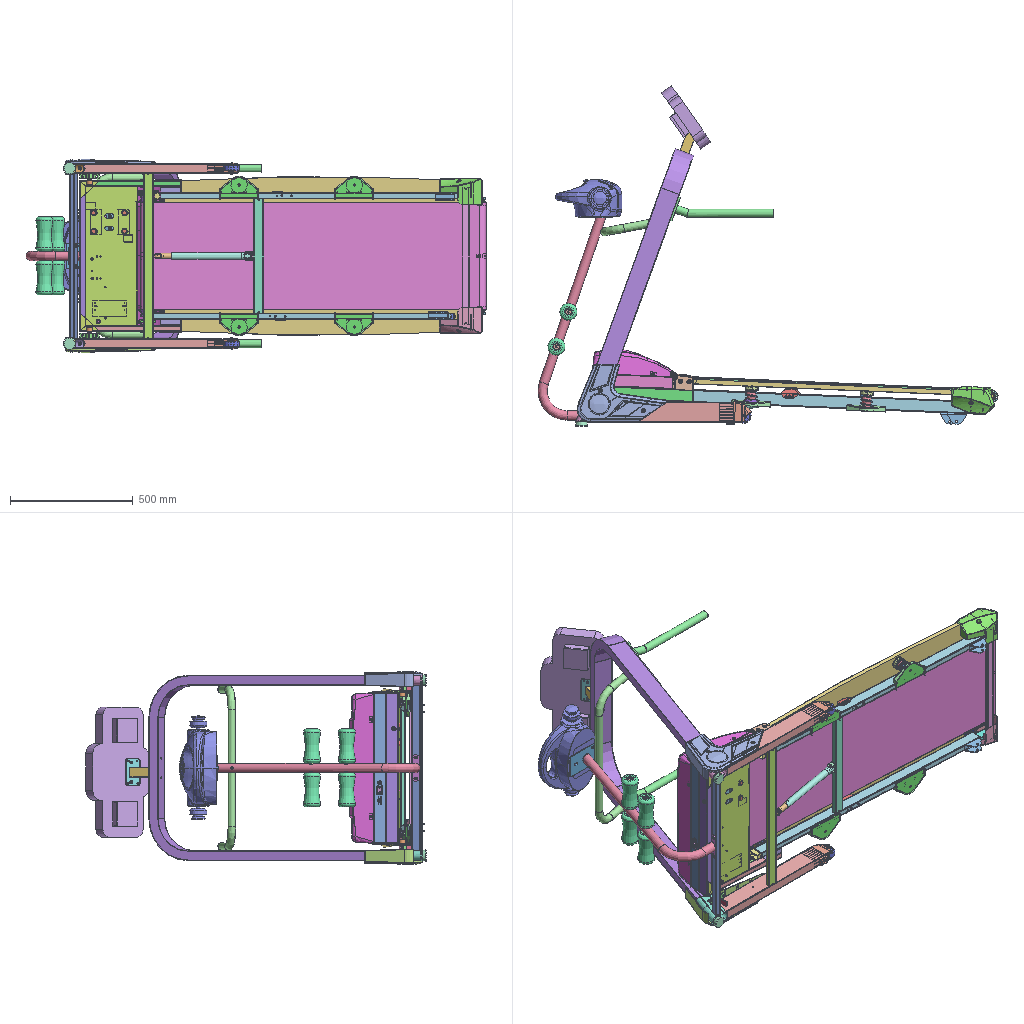Assembly | STEP file | 111 different items | 206 placed | box 1875 x 1387 x 788 mm
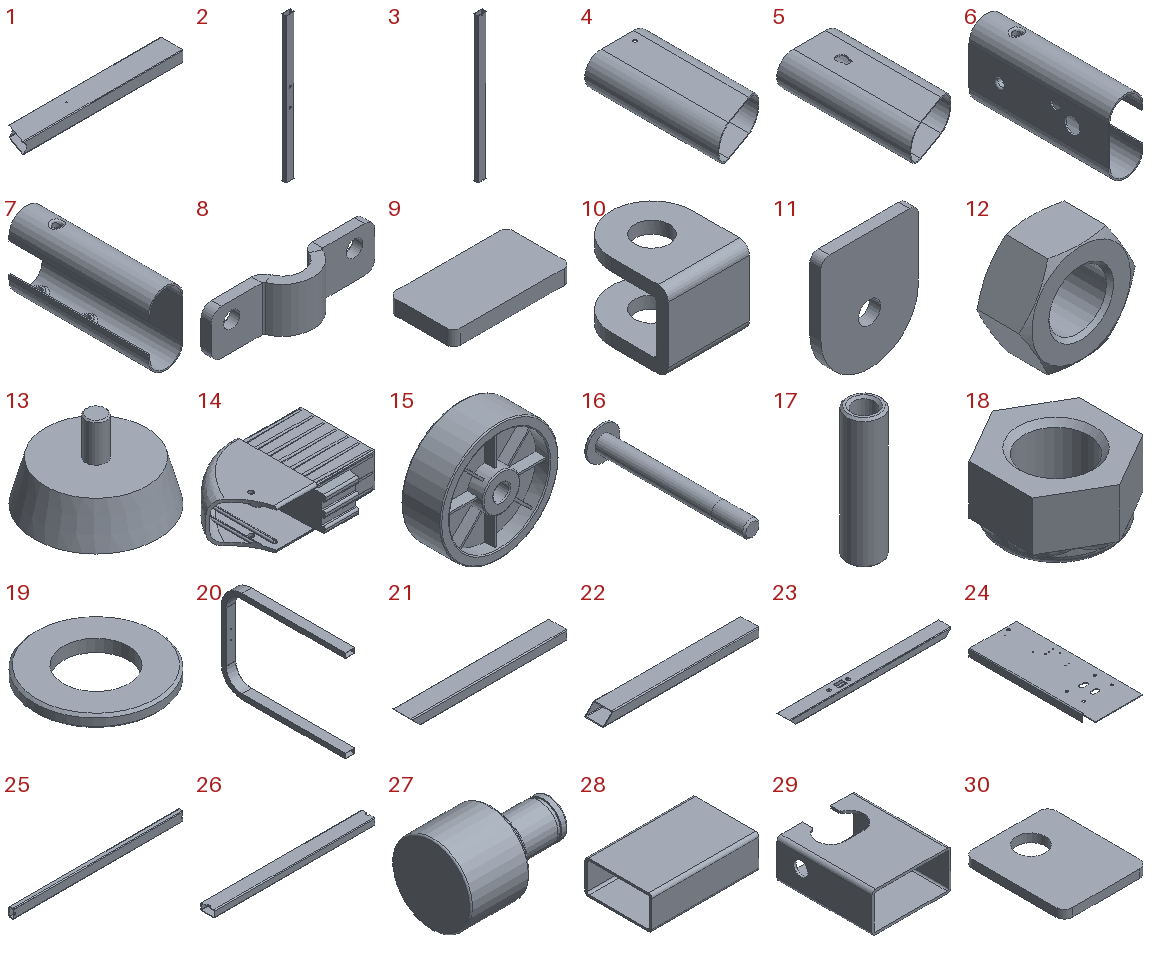Parts list (item | name | quantity | parent item | size | volume):
1 | 6100101 | x2 | in 6100100 | 569.929 x 80 x 40 mm | 191502 mm3
2 | 6100102 | x1 | in 6100100 | 40 x 20 x 675 mm | 111794 mm3
3 | 6100103 | x1 | in 6100100 | 40 x 20 x 675 mm | 112265 mm3
4 | 6100104L | x1 | in 6100100 | 80 x 165 x 40 mm | 45327 mm3
5 | 6100104R | x1 | in 6100100 | 80 x 165 x 40 mm | 45123 mm3
6 | 6100105L | x1 | in 6100100 | 36 x 145 x 76 mm | 34893 mm3
7 | 6100105R | x1 | in 6100100 | 36 x 145 x 76 mm | 34904 mm3
8 | 6100106 | x2 | in 6100100 | 80 x 15 x 22 mm | 9096 mm3
9 | 6100107 | x2 | in 6100100 | 40 x 22 x 5 mm | 4373 mm3
10 | PN_0023_default | x1 | in 6100100 | 20 x 24 x 19 mm | 3011 mm3
11 | 6100109 | x2 | in 6100100 | 35 x 4 x 42.5 mm | 5208 mm3
12 | N108078 | x8 | in 6100100, 6100500, 6101300 | 16.166 x 7 x 14 mm | 821.972 mm3
13 | 6100101W | x2 | in 6100100Z | 48.593 x 48.593 x 32 mm | 27204 mm3
14 | PN_0017_default | x2 | in 6100102LWZ, 6100102RWZ | 130 x 91 x 40 mm | 95148 mm3
15 | PN_0009_default | x2 | in 6100102LWZ, 6100102RWZ | 60 x 22 x 60 mm | 32782 mm3
16 | SD10545 | x2 | in 6100102LWZ, 6100102RWZ | 10 x 47.433 x 10 mm | 991.806 mm3
17 | 6100104W | x2 | in 6100102LWZ, 6100102RWZ | 8.2 x 8.2 x 31 mm | 968.239 mm3
18 | PN_0014 | x2 | in 6100102LWZ, 6100102RWZ | 8.5 x 9.815 x 5.1 mm | 204.852 mm3
19 | PN_0002 | x2 | in 6100102LWZ, 6100102RWZ | 10 x 10 x 1 mm | 55.238 mm3
20 | 6100201R | x1 | in 610 | 80 x 1020 x 755 mm | 1103888 mm3
21 | 6100501L | x1 | in 6100500 | 410 x 50 x 25 mm | 84495 mm3
22 | 6100501R | x1 | in 6100500 | 410 x 50 x 25 mm | 84495 mm3
23 | 6100502 | x1 | in 6100500 | 613 x 50 x 25 mm | 116984 mm3
24 | PN_0005_default | x1 | in 6100500 | 210 x 564 x 33 mm | 393745 mm3
25 | 6100504 | x1 | in 6100500 | 555 x 15 x 30 mm | 67311 mm3
26 | 6100505 | x1 | in 6100500 | 465 x 40 x 20 mm | 77302 mm3
27 | 6100506 | x2 | in 6100500 | 38 x 25.4 x 25.4 mm | 12200 mm3
28 | 6100507 | x2 | in 6100500 | 80 x 50 x 25 mm | 17005 mm3
29 | 6100508 | x1 | in 6100500 | 50 x 60 x 25 mm | 11554 mm3
30 | 6100509 | x1 | in 6100500 | 50 x 60 x 5 mm | 13731 mm3
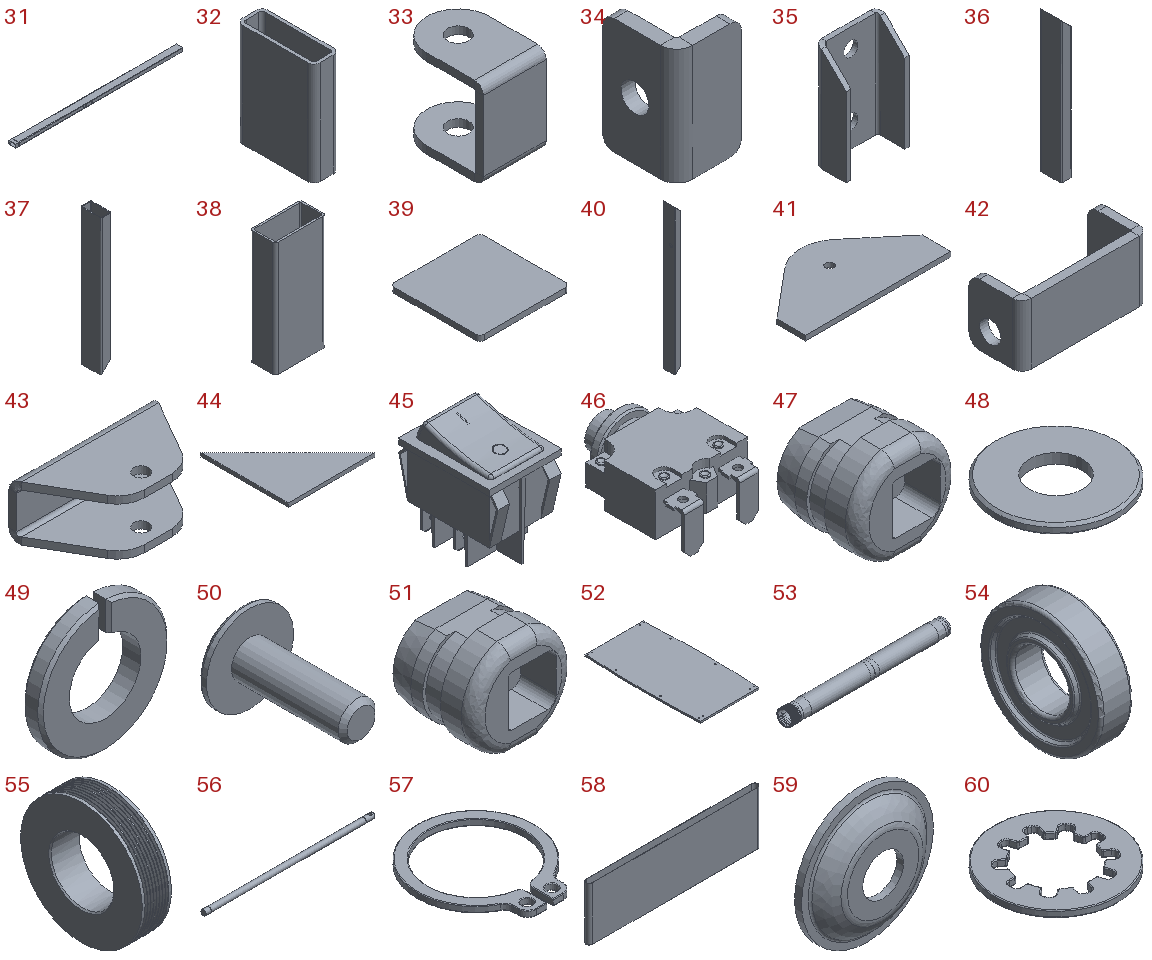31 | 6100510 | x2 | in 6100500 | 1235 x 50 x 25 mm | 261105 mm3
32 | 6100511 | x2 | in 6100500 | 10 x 30 x 40 mm | 3453 mm3
33 | 6100512 | x1 | in 6100500 | 25 x 35 x 35 mm | 6553 mm3
34 | 6100513 | x4 | in 6100500 | 14 x 16 x 25 mm | 1860 mm3
35 | 6100514 | x4 | in 6100500 | 40 x 20 x 67 mm | 13099 mm3
36 | 6100515 | x1 | in 6100500 | 25 x 50 x 334 mm | 67995 mm3
37 | 6100516 | x1 | in 6100500 | 25 x 50 x 334 mm | 67613 mm3
38 | 6100517 | x2 | in 6100500 | 40 x 20 x 90 mm | 14984 mm3
39 | 6100518 | x2 | in 6100500 | 50 x 50 x 3 mm | 7484 mm3
40 | 6100519 | x1 | in 6100500 | 25 x 50 x 613 mm | 123960 mm3
41 | PN_0001_default | x4 | in 6100500 | 150 x 80 x 5 mm | 44151 mm3
42 | 6100521 | x2 | in 6100500 | 60 x 25 x 29 mm | 10869 mm3
43 | 6100522 | x2 | in 6100500 | 80 x 44.5 x 31 mm | 26494 mm3
44 | 6100523 | x2 | in 6100500 | 70 x 70 x 3 mm | 7350 mm3
45 | EP002 | x1 | in 6100500Z | 25 x 34.5 x 34.784 mm | 14567 mm3
46 | EC002 | x1 | in 6100500Z | 29.3 x 39.3 x 19.65 mm | 10331 mm3
47 | PN_0024_default | x1 | in 6100500Z | 17 x 14 x 16 mm | 1519 mm3
48 | PN_0012 | x4 | in 6100500Z | 9.8 x 9.8 x 0.8 mm | 48.045 mm3
49 | W204009 | x4 | in 6100500Z | 9.2 x 1.3 x 9.193 mm | 57.255 mm3
50 | SD10412 | x4 | in 6100500Z | 9.4 x 14.503 x 9.4 mm | 245.335 mm3
51 | PN_0025_default | x1 | in 6100500Z | 17 x 14 x 16 mm | 1519 mm3
52 | DECAK 601 | x1 | in 6100500Z | 645 x 1220 x 18 mm | 13904736 mm3
53 | 610B0701 | x1 | in 610B0700Z | 515 x 50 x 50 mm | 253052 mm3
54 | PL6203ZZA_default | x4 | in 610B0700Z, 610B0800Z | 11 x 42 x 42 mm | 10581 mm3
55 | PN_0019_default | x1 | in 610B0700Z | 23 x 96 x 96 mm | 114860 mm3
56 | 610B0702 | x1 | in 610B0700Z | 565 x 17 x 17 mm | 128554 mm3
57 | PN_0018 | x4 | in 610B0700Z, 610B0800Z | 19 x 21.5 x 1 mm | 101.865 mm3
58 | RUBE 601 | x1 | in 6100500Z | 1411 x 53.2 x 440 mm | 2026187 mm3
59 | PN_0021_default | x1 | in 6100500Z | 21 x 3.607 x 21 mm | 386.807 mm3
60 | PN_0022 | x1 | in 6100500Z | 15 x 15 x 0.8 mm | 82.689 mm3
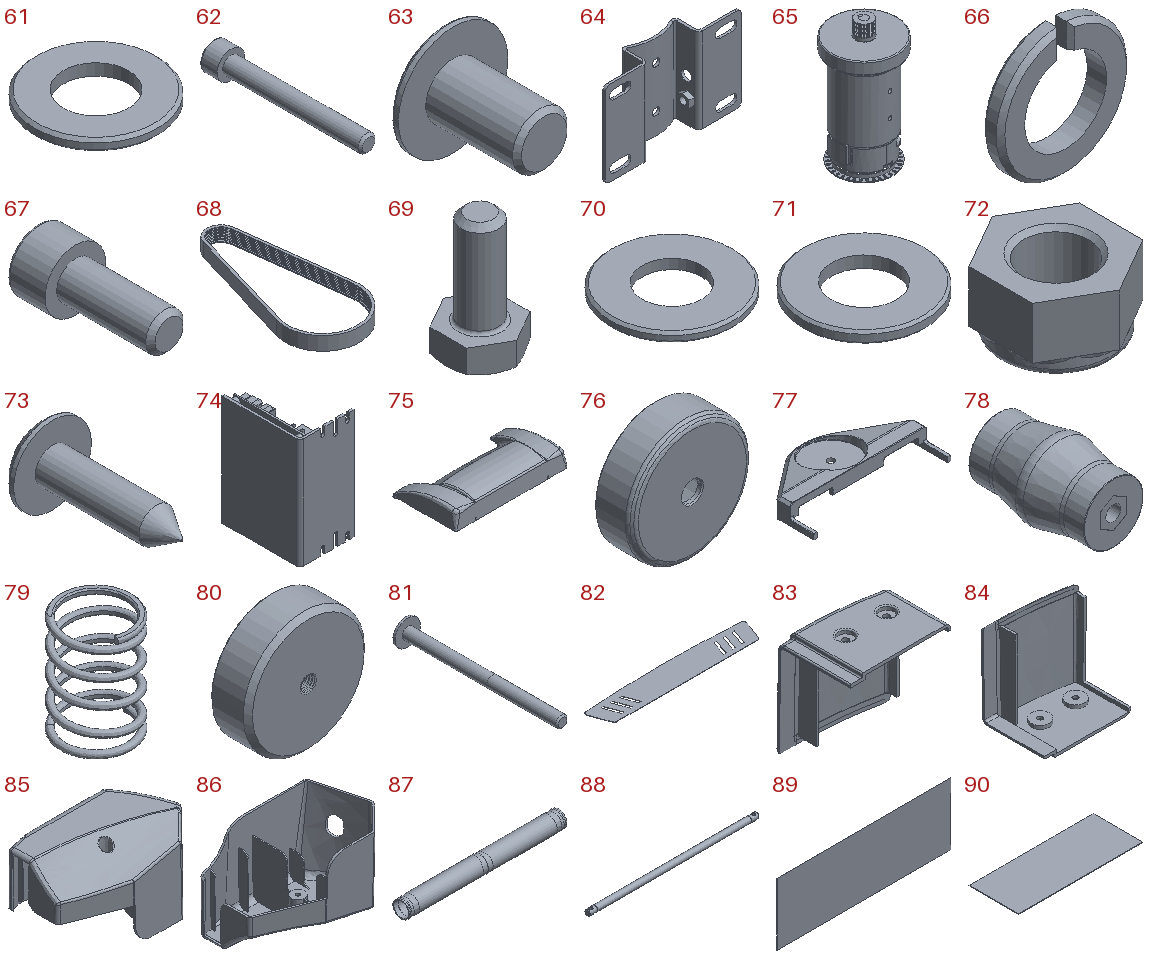61 | PN_0007 | x2 | in 6100500Z | 17 x 17 x 1.6 mm | 252.969 mm3
62 | SA10865 | x1 | in 6100500Z | 13 x 73 x 13 mm | 4160 mm3
63 | SD10610 | x3 | in 6100500Z | 12 x 12.964 x 12 mm | 479.053 mm3
64 | 6100601 | x1 | in 6100600Z | 160 x 30 x 100 mm | 59957 mm3
65 | MOTOR 602 | x1 | in 6100600Z | - | -
66 | W208016 | x2 | in 6100600Z | 13.5 x 2 x 13.481 mm | 158.687 mm3
67 | SA10820 | x2 | in 6100600Z | 13 x 28 x 13 mm | 1898 mm3
68 | DE200J601 | x1 | in 6100500Z | 99 x 216 x 18 mm | 21820 mm3
69 | SI1025_M10 | x4 | in 6100500Z | 17 x 19.6 x 32 mm | 3678 mm3
70 | PN_0008 | x4 | in 6100500Z | 25 x 25 x 2 mm | 736.18 mm3
71 | PN_0004 | x4 | in 6100500Z | 21 x 21 x 2 mm | 492.233 mm3
72 | N210095 | x4 | in 6100500Z | 17 x 19.63 x 10.5 mm | 1722 mm3
73 | SD20415 | x1 | in 6100500Z | 9 x 17.646 x 9 mm | 255.973 mm3
74 | ZYXK6.1012.V1.1 | x1 | in 6100500Z | 67.5 x 97.5 x 137.5 mm | 163388 mm3
75 | 96L | x1 | in 6100500Z | - | -
76 | PN_0026_default | x1 | in 6100500Z | 52 x 16 x 52 mm | 11242 mm3
77 | PN_0013_default | x4 | in 6100500Z | 160 x 95 x 22 mm | 49068 mm3
78 | PN_0016_default | x4 | in 6100500Z | 40 x 62 x 40 mm | 28151 mm3
79 | PN_0006_default | x4 | in 6100500Z | - | 11391 mm3
80 | PN_0003_default | x4 | in 6100500Z | 52 x 16 x 52 mm | 16645 mm3
81 | PN_0020 | x1 | in 6100500Z | 18 x 114.451 x 18 mm | 6223 mm3
82 | ZHD 500.75 | x2 | in 6100500Z | 531.222 x 88.107 x 1 mm | 40969 mm3
83 | HGL | x1 | in 6100500Z | 86.869 x 62.947 x 84.977 mm | 34701 mm3
84 | HGR | x1 | in 6100500Z | 86.869 x 62.947 x 84.977 mm | 34701 mm3
85 | HHJL | x1 | in 6100500Z | 176.285 x 110 x 105 mm | 139375 mm3
86 | HHJR | x1 | in 6100500Z | 176.285 x 110 x 105.001 mm | 141241 mm3
87 | 610B0801 | x1 | in 610B0800Z | 475 x 50 x 50 mm | 237316 mm3
88 | 610B0802 | x1 | in 610B0800Z | 523 x 17 x 17 mm | 116777 mm3
89 | Polyester film | x1 | in 6100500Z | 1200 x 0.25 x 430 mm | 129000 mm3
90 | Vibration-damping sponge | x1 | in 6100500Z | 1080 x 430 x 5 mm | 2322000 mm3
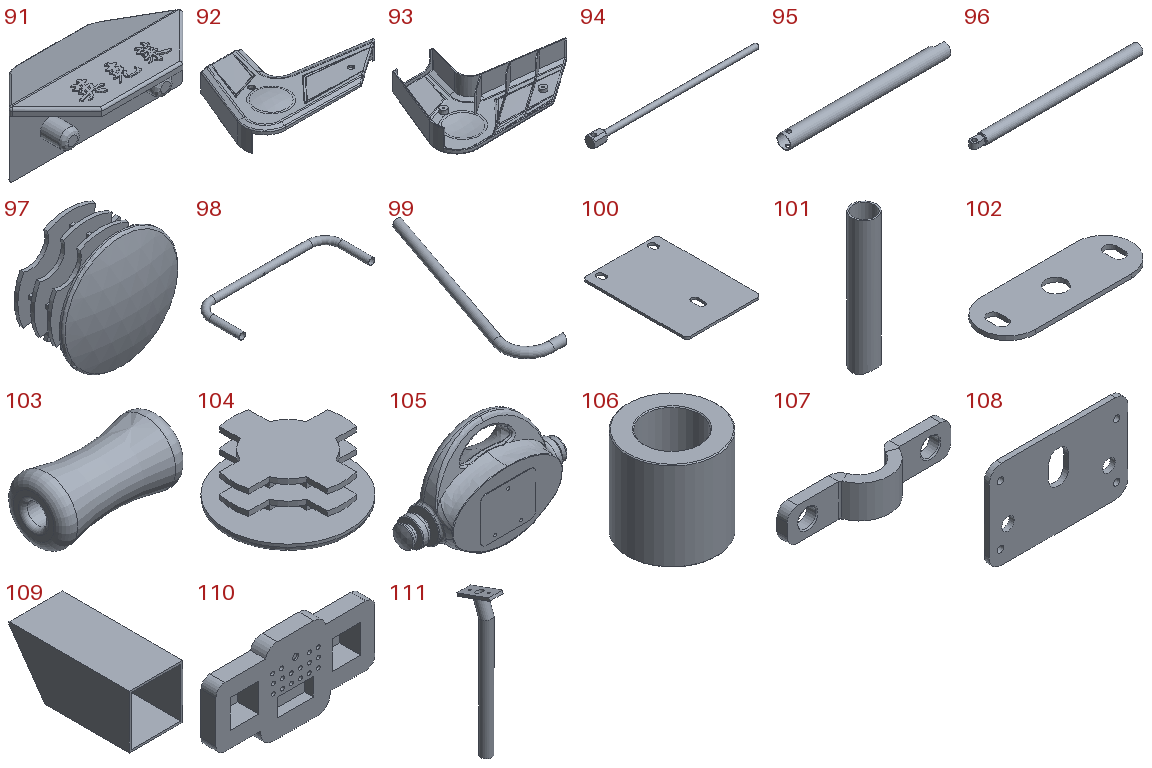91 | DECH07 | x2 | in 6100500Z | 74.172 x 40 x 28.5 mm | 30644 mm3
92 | BLZHT2-L | x1 | in 610 | 369.553 x 235 x 62.57 mm | 247383 mm3
93 | BLZHT2-R | x1 | in 610 | 369.553 x 235 x 62.57 mm | 247381 mm3
94 | GAS SHOCK 609S | x1 | in 610 | 353.5 x 20 x 20 mm | 34694 mm3
95 | GAS SHOCK 610W | x1 | in 610 | 330 x 28 x 28 mm | 39789 mm3
96 | GAS SHOCK 609X | x1 | in 610 | 359 x 22 x 22 mm | 94119 mm3
97 | 6101301W | x2 | in 6101300Z | 31.8 x 17.071 x 31.8 mm | 4059 mm3
98 | 6101301 | x1 | in 6101300 | 671.8 x 245.9 x 31.8 mm | 146844 mm3
99 | 6101401 | x1 | in 6101400 | 276.919 x 826.178 x 38.1 mm | 166528 mm3
100 | 6101402 | x1 | in 6101400 | 100 x 140 x 3 mm | 40958 mm3
101 | 6101403 | x4 | in 6101400 | 25.4 x 25.4 x 140 mm | 15577 mm3
102 | PN_0011_default | x1 | in 6101400 | 110 x 40 x 3 mm | 10934 mm3
103 | 6101402W | x4 | in 6101400Z | 140 x 70 x 70 mm | 348651 mm3
104 | 6101403W | x4 | in 6101400Z | 25.4 x 25.4 x 10 mm | 1636 mm3
105 | 6101404W | x1 | in 6101400Z | 430 x 154.443 x 270 mm | 5728271 mm3
106 | PN_0015_default | x2 | in 610 | 20 x 20 x 20 mm | 3941 mm3
107 | PN_0010_default | x2 | in 610 | 80 x 15 x 16 mm | 6317 mm3
108 | 10 | x1 | in Table header | 110 x 4 x 70 mm | 28070 mm3
109 | 101 | x1 | in Table header | 40 x 90 x 40 mm | 17766 mm3
110 | 111 | x1 | in 610 | 530 x 80 x 280 mm | 5097717 mm3
111 | 1112 | x2 | in 610 | 40 x 96.705 x 421.603 mm | 104269 mm3
Placements (level | parent | child | x y z in mm | rotation matrix by rows):
1 | 610 | 6100100Z | 350.123 -44.677 -99.489 | 1 0 0 0 1 0 0 0 1
2 | 6100100Z | 6100100 | -0.0 -0.0 -0.0 | 1 0 0 0 1 0 0 0 1
3 | 6100100 | 6100101 | -0.0 -0.0 -0.0 | 1 0 0 0 1 0 0 0 1
3 | 6100100 | 6100101 | -0.0 -0.0 -715.0 | 1 0 0 0 1 0 0 0 1
3 | 6100100 | 6100102 | -614.19 24.779 -357.5 | -0.342 0.9397 0 -0.9397 -0.342 0 0 0 1
3 | 6100100 | 6100103 | -300.0 0.0 -357.5 | 1 0 0 0 1 0 0 0 1
3 | 6100100 | 6100104L | -606.905 -13.681 -0.0 | 0.9397 0.342 0 -0.342 0.9397 0 0 0 1
3 | 6100100 | 6100104R | -606.905 -13.681 -715.0 | 0.9397 0.342 0 -0.342 0.9397 0 0 0 1
3 | 6100100 | 6100105L | -592.352 84.78 -0.0 | 0 0.342 0.9397 0 0.9397 -0.342 -1 0 -0
3 | 6100100 | 6100105R | -592.352 84.78 -715.0 | 0 0.342 0.9397 0 0.9397 -0.342 -1 0 -0
3 | 6100100 | 6100106 | -540.0 75.0 -684.0 | 1 0 0 0 1 0 0 0 1
3 | 6100100 | 6100106 | -540.0 75.0 -31.0 | -1 0 0 0 1 0 0 0 -1
3 | 6100100 | 6100107 | -540.5 46.446 -686.228 | 0 0 -1 -1 0 0 0 1 -0
3 | 6100100 | 6100107 | -540.5 46.446 -33.228 | 0 0 -1 -1 0 0 0 1 -0
3 | 6100100 | PN_0023_default | -280.0 10.0 -357.5 | 0 1 0 -1 0 0 0 0 1
3 | 6100100 | 6100109 | -621.209 3.0 -0.0 | 0 0 1 0 1 0 -1 0 0
3 | 6100100 | 6100109 | -621.209 3.0 -715.0 | 0 0 1 0 1 0 -1 0 0
3 | 6100100 | N108078 | -592.107 16.742 -315.0 | 0.2731 -0.9397 0.2058 0.7505 0.342 0.5655 -0.6018 0 0.7986
3 | 6100100 | N108078 | -592.107 16.742 -400.0 | 0.2731 -0.9397 0.2058 0.7505 0.342 0.5655 -0.6018 0 0.7986
2 | 6100100Z | 6100101W | -621.209 -0.0 -0.0 | 1 0 0 0 0 1 0 -1 0
2 | 6100100Z | 6100101W | -621.209 -0.0 -715.0 | 1 0 0 0 0 1 0 -1 0
2 | 6100100Z | 6100102LWZ | 70.0 80.0 20.0 | -1 0 0 0 1 0 0 0 -1
3 | 6100102LWZ | PN_0017_default | -0.0 -0.0 -0.0 | 1 0 0 0 1 0 0 0 1
3 | 6100102LWZ | PN_0009_default | 30.0 -55.0 9.0 | 0.9716 0 -0.2367 -0.2367 0 -0.9716 0 1 -0
3 | 6100102LWZ | SD10545 | 30.0 -55.0 -0.0 | 1 0 0 0 0 1 0 -1 -0
3 | 6100102LWZ | 6100104W | 30.0 -55.0 35.5 | 1 0 0 0 1 0 0 0 1
3 | 6100102LWZ | PN_0014 | 30.0 -55.0 44.8 | -0.9237 -0.383 0 -0.383 0.9237 0 0 0 -1
3 | 6100102LWZ | PN_0002 | 30.0 -55.0 40.0 | 1 0 0 0 1 0 0 0 1
2 | 6100100Z | 6100102RWZ | 70.0 80.0 -695.0 | -1 0 0 0 1 0 0 0 -1
3 | 6100102RWZ | PN_0017_default | -0.0 -0.0 -0.0 | 1 0 0 0 1 0 0 0 1
3 | 6100102RWZ | PN_0009_default | 30.0 -55.0 9.0 | 0.9716 0 -0.2367 -0.2367 0 -0.9716 0 1 -0
3 | 6100102RWZ | SD10545 | 30.0 -55.0 40.0 | -0.9237 0 -0.383 -0.383 0 0.9237 0 1 -0
3 | 6100102RWZ | 6100104W | 30.0 -55.0 35.5 | 1 0 0 0 1 0 0 0 1
3 | 6100102RWZ | PN_0014 | 30.0 -55.0 -4.8 | 1 0 0 0 1 0 0 0 1
3 | 6100102RWZ | PN_0002 | 30.0 -55.0 0.0 | -0.9237 -0.383 0 -0.383 0.9237 0 0 0 -1
1 | 610 | 6100201R | -200.348 96.691 -814.489 | -0.9397 0.342 0 0.342 0.9397 0 0 0 -1
1 | 610 | 6100500Z | -133.133 138.176 -146.531 | 0.9991 0.04155 0 -0.04155 0.9991 0 0 0 1
2 | 6100500Z | 6100500 | -0.0 -0.0 -0.0 | 1 0 0 0 1 0 0 0 1
3 | 6100500 | 6100501L | 112.255 -64.436 -15.459 | 1 0 0 0 1 0 0 0 1
3 | 6100500 | 6100501R | 112.255 -64.436 -605.459 | 1 0 0 0 1 0 0 0 1
3 | 6100500 | 6100502 | -80.245 -14.436 -310.459 | 0 0 -1 0 1 0 1 0 0
3 | 6100500 | PN_0005_default | -67.745 -86.436 -310.459 | -1 0 0 0 0 -1 0 -1 0
3 | 6100500 | 6100504 | 1482.255 -76.936 -310.459 | 0 0 1 0 1 0 -1 0 -0
3 | 6100500 | 6100505 | 637.255 -79.436 -310.459 | 0 -1 0 0 0 -1 1 0 0
3 | 6100500 | 6100506 | -52.745 -105.136 -600.459 | 0 0 -1 0 -1 0 -1 0 -0
3 | 6100500 | 6100507 | 277.255 -64.436 -40.459 | 1 0 0 0 1 0 0 0 1
3 | 6100500 | 6100508 | 177.255 -27.436 -580.459 | 1 0 0 0 1 0 0 0 1
3 | 6100500 | 6100509 | 177.255 -57.436 -32.959 | 1 0 0 0 1 0 0 0 1
3 | 6100500 | 6100510 | 829.755 -64.436 -65.459 | 1 0 0 0 -1 0 0 0 -1
3 | 6100500 | 6100510 | 802.255 -64.436 -555.459 | 1 0 0 0 1 0 0 0 1
3 | 6100500 | 6100511 | 104.255 -137.337 -252.977 | 0 0 1 -1 0 0 0 -1 0
3 | 6100500 | 6100511 | -47.745 -25.535 -120.977 | 0 0 -1 1 0 0 0 -1 -0
3 | 6100500 | 6100512 | 617.255 -81.936 -310.459 | 0 -1 0 1 0 0 0 0 1
3 | 6100500 | 6100513 | 154.255 10.564 -614.959 | 0 0 -1 0 1 0 1 0 0
3 | 6100500 | 6100513 | -92.745 10.564 -112.959 | 1 0 0 0 1 0 0 0 1
3 | 6100500 | 6100513 | 154.255 10.564 -5.959 | 0 0 1 0 1 0 -1 0 0
3 | 6100500 | 6100513 | -92.745 10.564 -507.959 | 1 0 0 0 1 0 0 0 1
3 | 6100500 | 6100514 | 1413.255 -54.436 -42.959 | 1 0 0 0 1 0 0 0 1
3 | 6100500 | 6100514 | 1413.255 -54.436 -577.959 | -1 0 0 0 1 0 0 0 -1
3 | 6100500 | 6100514 | 268.255 -54.436 -37.959 | -1 0 0 0 1 0 0 0 -1
3 | 6100500 | 6100514 | 268.255 -54.436 -582.959 | 1 0 0 0 1 0 0 0 1
3 | 6100500 | 6100515 | 241.255 -14.436 -605.459 | 0 0 -1 0 1 0 1 0 -0
3 | 6100500 | 6100516 | -92.745 -14.436 -15.459 | 0 0 1 0 1 0 -1 0 0
3 | 6100500 | 6100517 | 1433.255 -49.436 -42.959 | 0 0 1 -1 0 0 0 -1 0
3 | 6100500 | 6100517 | 1433.255 -49.436 -577.959 | 0 0 1 -1 0 0 0 -1 0
3 | 6100500 | 6100518 | 320.255 -64.436 -27.959 | 0 0 -1 0 1 0 1 0 0
3 | 6100500 | 6100518 | 317.255 -64.436 -592.959 | 0 0 1 0 1 0 -1 0 -0
3 | 6100500 | 6100519 | -80.245 -64.436 -616.959 | 1 0 0 0 1 0 0 0 1
3 | 6100500 | PN_0001_default | 557.255 -89.436 -70.959 | 1 0 0 0 0 -1 0 1 0
3 | 6100500 | PN_0001_default | 557.255 -94.436 -549.959 | 1 0 0 0 0 1 0 -1 -0
3 | 6100500 | PN_0001_default | 1027.255 -89.436 -70.959 | 1 0 0 0 0 -1 0 1 0
3 | 6100500 | PN_0001_default | 1027.255 -94.436 -549.959 | 1 0 0 0 0 1 0 -1 -0
3 | 6100500 | 6100521 | 1483.255 -29.436 -54.459 | 1 0 0 0 1 0 0 0 1
3 | 6100500 | 6100521 | 1483.255 -29.436 -566.459 | -1 0 0 0 1 0 0 0 -1
3 | 6100500 | 6100506 | -52.745 -105.136 -20.459 | 0 0 1 0 -1 0 1 0 -0
3 | 6100500 | 6100522 | 1369.755 -133.936 -552.459 | 1 0 0 0 1 0 0 0 1
3 | 6100500 | 6100522 | 1397.255 -133.936 -68.459 | 1 0 0 0 1 0 0 0 1
3 | 6100500 | 6100523 | -71.68 -92.436 -597.95 | 0 1 0 0 0 1 1 0 0
3 | 6100500 | N108078 | 268.255 -25.936 -57.959 | 1 0 0 0 1 0 0 0 1
3 | 6100500 | N108078 | 268.255 -25.936 -562.959 | 1 0 0 0 1 0 0 0 1
3 | 6100500 | N108078 | 1413.255 -25.936 -557.959 | 1 0 0 0 1 0 0 0 1
3 | 6100500 | N108078 | 1413.255 -25.936 -62.959 | 1 0 0 0 1 0 0 0 1
3 | 6100500 | 6100523 | -71.68 -89.436 -22.968 | 0 1 0 0 0 -1 -1 0 0
3 | 6100500 | 6100507 | 277.255 -64.436 -580.459 | 1 0 0 0 1 0 0 0 1
2 | 6100500Z | EP002 | -92.745 -14.186 -399.709 | 0 0 -1 -1 0 0 0 1 0
2 | 6100500Z | EC002 | -35.465 -21.336 -400.294 | 0 -1 0 0 0 -1 1 0 0
2 | 6100500Z | PN_0024_default | -98.245 -14.524 -371.359 | 0 1 0 -1 0 0 0 0 1
2 | 6100500Z | PN_0012 | 12.255 -82.636 -437.459 | 1 0 0 0 0 -1 0 1 -0
2 | 6100500Z | PN_0012 | -42.745 -86.436 -322.459 | 0.9885 -0.1514 0 0 0 1 -0.1514 -0.9885 0
2 | 6100500Z | PN_0012 | -42.745 -86.436 -402.459 | 1 0 0 0 0 1 0 -1 0
2 | 6100500Z | PN_0012 | 12.255 -84.436 -562.459 | 0.8986 -0.4389 0 0 0 1 -0.4389 -0.8986 0
2 | 6100500Z | W204009 | 12.255 -82.636 -437.459 | -0.2314 0 0.9729 0 1 0 -0.9729 0 -0.2314
2 | 6100500Z | W204009 | -42.745 -84.336 -322.459 | 0.9816 0 -0.1911 0 -1 0 -0.1911 0 -0.9816
2 | 6100500Z | W204009 | -42.745 -84.336 -402.459 | 1 0 0 0 -1 0 0 0 -1
2 | 6100500Z | W204009 | 12.255 -82.336 -562.459 | 1 0 0 0 -1 0 0 0 -1
2 | 6100500Z | SD10412 | -42.745 -84.336 -402.459 | -0.8802 0 -0.4746 0 1 0 0.4746 0 -0.8802
2 | 6100500Z | SD10412 | -42.745 -84.336 -322.459 | 0.9884 0 0.152 0 1 0 -0.152 0 0.9884
2 | 6100500Z | SD10412 | 12.255 -81.336 -437.459 | 0.8688 0 -0.4951 0 1 0 0.4951 0 0.8688
2 | 6100500Z | SD10412 | 12.255 -82.336 -562.459 | 0.2995 0 -0.9541 0 1 0 0.9541 0 0.2995
2 | 6100500Z | PN_0025_default | -17.579 -94.936 -577.464 | -0.9995 0 -0.03043 0 1 0 0.03043 0 -0.9995
2 | 6100500Z | DECAK 601 | 859.255 -5.436 -310.459 | 0 -1 0 0 0 1 -1 0 0
2 | 6100500Z | 610B0700Z | 177.255 -12.436 -311.159 | 0 0 1 0 1 0 -1 0 0
3 | 610B0700Z | 610B0701 | -0.0 0.0 -0.0 | 1 0 0 0 1 0 0 0 1
3 | 610B0700Z | PL6203ZZA_default | -269.0 9.5 -0.0 | 1 0 0 0 1 0 0 0 1
3 | 610B0700Z | PL6203ZZA_default | 235.0 9.5 -0.0 | 1 0 0 0 1 0 0 0 1
3 | 610B0700Z | PN_0019_default | -246.0 0.0 -0.0 | -1 0 0 0 0.5305 0.8477 0 0.8477 -0.5305
3 | 610B0700Z | 610B0702 | -34.7 0.0 -0.0 | 1 0 0 0 1 0 0 0 1
3 | 610B0700Z | PN_0018 | 247.1 0.0 -0.0 | 0 0 -1 0 1 0 1 0 0
3 | 610B0700Z | PN_0018 | -270.1 0.0 -0.0 | 0 0 1 0 1 0 -1 0 0
2 | 6100500Z | RUBE 601 | 1425.752 -15.962 -310.459 | 1 0.001223 0 -0.001223 1 0 0 0 1
2 | 6100500Z | PN_0021_default | -22.745 -1.389 -15.959 | 1 0 0 0 1 0 0 0 1
2 | 6100500Z | PN_0022 | 151.455 -12.436 -577.959 | 0 0 1 0 1 0 -1 0 0
2 | 6100500Z | PN_0007 | 149.855 -12.436 -577.959 | 0 0 1 0 1 0 -1 0 0
2 | 6100500Z | SA10865 | 149.855 -12.436 -577.959 | 0 -1 0 1 0 0 0 0 1
2 | 6100500Z | SD10610 | 154.255 19.564 -2.959 | 0.9957 0 -0.09225 -0.09225 0 -0.9957 0 1 0
2 | 6100500Z | SD10610 | -95.745 19.564 -112.959 | 0 -1 0 1 0 0 0 0 1
2 | 6100500Z | SD10610 | 154.255 19.564 -617.959 | -0.9199 0 0.3922 -0.3922 0 -0.9199 0 -1 -0
2 | 6100500Z | 6100600Z | 29.378 -81.436 -172.459 | -1 0 0 0 1 0 0 0 -1
3 | 6100600Z | 6100601 | -0.0 0.0 -0.0 | 1 0 0 0 1 0 0 0 1
3 | 6100600Z | MOTOR 602 | -0.0 75.0 2.8 | -1 0 0 0 1 0 0 0 -1
3 | 6100600Z | W208016 | -0.0 15.0 25.0 | 1 0 -1e-06 0 1 0 1e-06 0 1
3 | 6100600Z | W208016 | -0.0 15.0 -25.0 | 1 0 -1e-06 0 1 0 1e-06 0 1
3 | 6100600Z | SA10820 | -0.0 15.0 25.0 | 0.02966 0 -0.9996 0 -1 0 -0.9996 0 -0.02966
3 | 6100600Z | SA10820 | -0.0 15.0 -25.0 | -0.9974 0 -0.07138 0 -1 0 -0.07138 0 0.9974
2 | 6100500Z | DE200J601 | 385.699 -534.85 -53.659 | -0.1223 -0.9925 0 -0.9925 0.1223 0 0 0 -1
2 | 6100500Z | SI1025_M10 | -35.245 -96.436 -134.959 | 0.7133 -0.7008 0 0 0 1 -0.7008 -0.7133 -0
2 | 6100500Z | SI1025_M10 | -35.245 -96.436 -209.959 | -0.1244 0.9922 0 0 0 1 0.9922 0.1244 -0
2 | 6100500Z | SI1025_M10 | 89.755 -96.436 -134.959 | 0.87 -0.493 0 0 0 1 -0.493 -0.87 -0
2 | 6100500Z | SI1025_M10 | 89.755 -96.436 -209.959 | 0.4078 -0.9131 0 0 0 1 -0.9131 -0.4078 0
2 | 6100500Z | PN_0008 | 89.755 -84.436 -209.959 | 1 0 0 0 0 -1 0 1 0
2 | 6100500Z | PN_0008 | 89.755 -84.436 -134.959 | 1 0 0 0 0 -1 0 1 0
2 | 6100500Z | PN_0008 | -35.245 -84.436 -209.959 | 1 0 0 0 0 -1 0 1 0
2 | 6100500Z | PN_0008 | -35.245 -84.436 -134.959 | 1 0 0 0 0 -1 0 1 0
2 | 6100500Z | PN_0004 | -35.245 -79.436 -134.959 | 1 0 0 0 0 -1 0 1 0
2 | 6100500Z | PN_0004 | 89.755 -79.436 -209.959 | 1 0 0 0 0 -1 0 1 0
2 | 6100500Z | PN_0004 | 89.755 -79.436 -134.959 | 1 0 0 0 0 -1 0 1 0
2 | 6100500Z | PN_0004 | -35.245 -79.436 -209.959 | 0.697 0.7171 0 0 0 -1 -0.7171 0.697 0
2 | 6100500Z | N210095 | -35.245 -71.436 -134.959 | 1 0 0 0 0 -1 0 1 0
2 | 6100500Z | N210095 | -35.245 -71.436 -209.959 | 1 0 0 0 0 -1 0 1 0
2 | 6100500Z | N210095 | 89.755 -71.436 -134.959 | 1 0 0 0 0 -1 0 1 0
2 | 6100500Z | N210095 | 89.755 -71.436 -209.959 | 1 0 0 0 0 -1 0 1 0
2 | 6100500Z | SD20415 | 1453.255 -44.436 -590.959 | -0.9853 0 0.1709 -0.1709 0 -0.9853 0 -1 0
2 | 6100500Z | ZYXK6.1012.V1.1 | 29.505 -86.436 -559.959 | 0 0 -1 0 1 0 1 0 0
2 | 6100500Z | 96L | 74.448 10.564 -310.459 | 0 1 0 0 0 1 1 0 0
2 | 6100500Z | PN_0026_default | 557.255 -85.436 -20.959 | 0.9852 0 -0.1715 0 1 0 0.1715 0 0.9852
2 | 6100500Z | PN_0013_default | 557.255 -95.436 -80.959 | -1 0 0 0 0 1 0 1 -0
2 | 6100500Z | PN_0016_default | 557.255 -52.436 -20.959 | 0.4311 0 -0.9023 0 1 0 0.9023 0 0.4311
2 | 6100500Z | PN_0006_default | 557.255 -16.536 -20.959 | 0.6547 -0.7559 0 0 0 -1 0.7559 0.6547 0
2 | 6100500Z | PN_0003_default | 557.255 -12.936 -20.959 | -0.7971 0 0.6039 0 -1 0 0.6039 0 0.7971
2 | 6100500Z | PN_0020 | -94.345 -72.436 -150.459 | 0 -1 0 0.5302 0 -0.8479 0.8479 0 0.5302
2 | 6100500Z | PN_0007 | -92.745 -72.436 -150.459 | 0 0 -1 -0.2254 0.9743 0 0.9743 0.2254 0
2 | 6100500Z | PN_0016_default | 557.255 -52.436 -599.959 | 0.4311 0 -0.9023 0 1 0 0.9023 0 0.4311
2 | 6100500Z | PN_0016_default | 1027.255 -53.01 -20.959 | 0.4311 0 -0.9023 0 1 0 0.9023 0 0.4311
2 | 6100500Z | PN_0016_default | 1027.255 -53.01 -599.959 | 0.4311 0 -0.9023 0 1 0 0.9023 0 0.4311
2 | 6100500Z | PN_0006_default | 557.255 -16.536 -599.959 | 0.6547 -0.7559 0 0 0 -1 0.7559 0.6547 0
2 | 6100500Z | PN_0006_default | 1027.255 -17.11 -20.959 | 0.6547 -0.7559 0 0 0 -1 0.7559 0.6547 0
2 | 6100500Z | PN_0006_default | 1027.255 -17.11 -599.959 | 0.6547 -0.7559 0 0 0 -1 0.7559 0.6547 0
2 | 6100500Z | PN_0003_default | 557.255 -12.936 -599.959 | -0.7971 0 0.6039 0 -1 0 0.6039 0 0.7971
2 | 6100500Z | PN_0003_default | 1027.255 -13.51 -20.959 | -0.7971 0 0.6039 0 -1 0 0.6039 0 0.7971
2 | 6100500Z | PN_0003_default | 1027.255 -13.51 -599.959 | -0.7971 0 0.6039 0 -1 0 0.6039 0 0.7971
2 | 6100500Z | PN_0013_default | 557.255 -95.436 -539.959 | 1 0 0 0 0 1 0 -1 -0
2 | 6100500Z | PN_0013_default | 1027.255 -96.01 -539.959 | 1 0 0 0 0 1 0 -1 -0
2 | 6100500Z | PN_0013_default | 1027.255 -96.01 -80.959 | -1 0 0 0 0 1 0 1 -0
2 | 6100500Z | ZHD 500.75 | 794.317 3.564 -591.214 | 1 0 0 0 0 1 0 -1 -0
2 | 6100500Z | ZHD 500.75 | 794.317 3.564 -29.703 | -1 0 0 0 0 1 0 1 -0
2 | 6100500Z | HGL | 283.428 -12.436 -39.459 | 1 0 0 0 1 0 0 0 1
2 | 6100500Z | HGR | 282.581 -10.335 -581.459 | 1 0 0 0 1 0 0 0 1
2 | 6100500Z | HHJL | 1450.255 20.564 -47.459 | 1 0 0 0 1 0 0 0 1
2 | 6100500Z | HHJR | 1450.255 20.564 -573.459 | 1 0 0 0 1 0 0 0 1
2 | 6100500Z | 610B0800Z | 1535.254 -14.096 -310.459 | 0 -0.06913 -0.9976 0 -0.9976 0.06913 -1 0 -0
3 | 610B0800Z | 610B0801 | 0.0 0.0 0.0 | 1 0 0 0 1 0 0 0 1
3 | 610B0800Z | 610B0802 | 0.0 0.0 0.0 | 1 0 0 0 1 0 0 0 1
3 | 610B0800Z | PL6203ZZA_default | -237.5 9.5 0.0 | 1 0 0 0 1 0 0 0 1
3 | 610B0800Z | PL6203ZZA_default | 226.5 9.5 0.0 | 1 0 0 0 1 0 0 0 1
3 | 610B0800Z | PN_0018 | 238.4 0.0 0.0 | 0 0 -1 0 1 0 1 0 0
3 | 610B0800Z | PN_0018 | -238.6 -0.0 0.0 | 0 0 1 0 1 0 -1 0 -0
2 | 6100500Z | Polyester film | 852.745 8.564 -314.015 | 1 0 0 0 1 0 0 0 1
2 | 6100500Z | Vibration-damping sponge | 859.255 8.564 -310.459 | 1 0 0 0 0 -1 0 1 -0
2 | 6100500Z | DECH07 | 712.255 -39.436 -77.759 | 1 0 0 0 1 0 0 0 1
2 | 6100500Z | DECH07 | 724.755 -39.436 -543.159 | -1 0 0 0 1 0 0 0 -1
1 | 610 | BLZHT2-L | 85.754 41.837 -98.489 | 1 0 0 0 1 0 0 0 1
1 | 610 | BLZHT2-R | 85.754 41.837 -815.489 | 1 0 0 0 1 0 0 0 1
1 | 610 | GAS SHOCK 609S | 438.011 28.106 -456.989 | -0.9846 0.1747 0 -0.1747 -0.9846 0 0 0 1
1 | 610 | GAS SHOCK 610W | 467.55 33.347 -456.989 | -0.9846 -0.1747 0 -0.1747 0.9846 0 0 0 -1
1 | 610 | GAS SHOCK 609X | 276.617 -0.5267 -456.989 | 0.9846 -0.1747 0 0.1747 0.9846 0 0 0 1
1 | 610 | 6101300Z | -17.785 821.073 -443.731 | 0 -0.9833 -0.1822 0 -0.1822 0.9833 -1 0 0
2 | 6101300Z | 6101301W | -306.741 -60.647 -60.297 | 0.985 0 0.1723 0 1 0 -0.1723 0 0.985
2 | 6101300Z | 6101301W | 333.259 -60.647 -60.297 | 0.8095 0 0.5871 0 1 0 -0.5871 0 0.8095
2 | 6101300Z | 6101300 | 58.763 25.746 -60.297 | 1 0 0 0 1 0 0 0 1
3 | 6101300 | 6101301 | -45.505 -82.821 0.0 | 1 0 0 0 1 0 0 0 1
3 | 6101300 | N108078 | -374.5 -62.821 0.0 | 0 1 0 -0.9975 0 0.07046 0.07046 0 0.9975
3 | 6101300 | N108078 | 283.49 -62.821 0.0 | 0 -1 0 -0.9975 0 -0.07046 0.07046 0 -0.9975
1 | 610 | 6101400Z | -302.905 321.975 -666.07 | 1 0 0 0 1 0 0 0 1
2 | 6101400Z | 6101400 | -82.682 -8.839 49.635 | 1 0 0 0 1 0 0 0 1
3 | 6101400 | 6101401 | 125.56 -332.214 159.445 | 1 0 0 0 1 0 0 0 1
3 | 6101400 | 6101402 | 170.56 474.914 159.445 | 0 1 0 0 0 1 1 0 -0
3 | 6101400 | 6101403 | 12.104 -51.264 244.793 | -0.9455 -0.3256 0 0.3256 -0.9455 0 0 0 1
3 | 6101400 | 6101403 | 60.939 90.564 244.793 | -0.9455 -0.3256 0 0.3256 -0.9455 0 0 0 1
3 | 6101400 | 6101403 | 60.939 90.564 74.097 | 0.9455 -0.3256 0 -0.3256 -0.9455 0 0 0 -1
3 | 6101400 | 6101403 | 12.104 -51.264 74.097 | 0.9455 -0.3256 0 -0.3256 -0.9455 0 0 0 -1
3 | 6101400 | PN_0011_default | 121.52 -333.034 159.445 | 0 0.342 -0.9397 0 0.9397 0.342 1 0 0
2 | 6101400Z | 6101402W | -21.743 81.725 298.13 | 0 0.0951 0.9955 0 0.9955 -0.0951 -1 0 0
2 | 6101400Z | 6101403W | -21.743 81.725 365.928 | -0.4687 -0.8834 0 -0.8834 0.4687 0 0 0 -1
2 | 6101400Z | 6101403W | -70.578 -60.103 365.928 | -0.4687 -0.8834 0 -0.8834 0.4687 0 0 0 -1
2 | 6101400Z | 6101403W | -70.578 -60.103 52.232 | -0.4628 0.8865 0 -0.8865 -0.4628 0 0 0 1
2 | 6101400Z | 6101403W | -21.743 81.725 52.232 | 0.9897 -0.143 0 0.143 0.9897 0 0 0 1
2 | 6101400Z | 6101402W | -21.743 81.725 120.13 | 0 0.0951 0.9955 0 0.9955 -0.0951 -1 0 0
2 | 6101400Z | 6101402W | -70.578 -60.103 298.13 | 0 0.0951 0.9955 0 0.9955 -0.0951 -1 0 0
2 | 6101400Z | 6101402W | -70.578 -60.103 120.13 | 0 0.0951 0.9955 0 0.9955 -0.0951 -1 0 0
2 | 6101400Z | 6101404W | 76.378 470.575 209.08 | 0 0 -1 0 1 0 1 0 -0
1 | 610 | PN_0015_default | -190.201 35.323 -794.489 | 0.4461 0.895 0 -0.895 0.4461 0 0 0 1
1 | 610 | PN_0015_default | -189.553 35.323 -139.489 | 0.7977 -0.6031 0 0.6031 0.7977 0 0 0 1
1 | 610 | PN_0010_default | -189.877 35.323 -788.489 | -1 0 0 0 -1 0 0 0 1
1 | 610 | PN_0010_default | -189.877 35.323 -141.489 | -1 0 0 0 -1 0 0 0 1
1 | 610 | Table header | 118.31 1229.081 -456.989 | 0 -0.8192 0.5736 0 -0.5736 -0.8192 1 0 -0
2 | Table header | 10 | -16.842 7.894 110.0 | 1 0 0 0 1 0 0 0 1
2 | Table header | 101 | -16.842 75.007 159.776 | 1 0 0 0 -0.8192 0.5736 0 -0.5736 -0.8192
1 | 610 | 111 | 167.633 1223.332 -473.831 | 0 -0.8192 0.5736 0 -0.5736 -0.8192 1 0 0
1 | 610 | 1112 | 189.54 810.014 -99.489 | 0 0 -1 0 1 0 1 0 0
1 | 610 | 1112 | 189.54 810.014 -814.489 | 0 0 -1 0 1 0 1 0 0